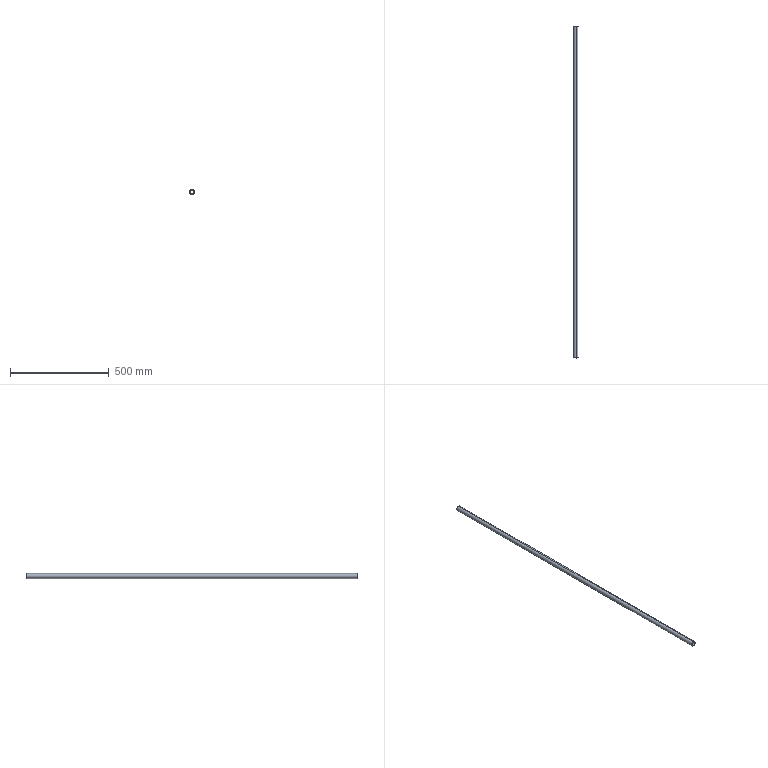Part | STEP file | PN_0046_Default<As Machined> | 1 solid | 6 faces | box 25.4 x 1683 x 25.4 mm | volume 334580 mm3 | cylinder 4 | plane 2 | commonest cylinder face diameters 19.8 x2 25.4 x2
STEP:
#1=CARTESIAN_POINT('',(0.,1683.,-9.9));
#2=VERTEX_POINT('',#1);
#3=CARTESIAN_POINT('',(0.,1683.,9.9));
#4=VERTEX_POINT('',#3);
#5=CARTESIAN_POINT('',(0.,1683.,0.));
#6=DIRECTION('',(0.,-1.,0.));
#7=AXIS2_PLACEMENT_3D('',#5,#6,$);
#8=CIRCLE('',#7,9.9);
#9=EDGE_CURVE('',#2,#4,#8,.F.);
#10=ORIENTED_EDGE('',*,*,#9,.T.);
#11=CARTESIAN_POINT('',(0.,0.,9.9));
#12=VERTEX_POINT('',#11);
#13=CARTESIAN_POINT('',(0.,1683.,9.9));
#14=DIRECTION('',(0.,-1.,0.));
#15=VECTOR('',#14,1.);
#16=LINE('',#13,#15);
#17=EDGE_CURVE('',#4,#12,#16,.T.);
#18=ORIENTED_EDGE('',*,*,#17,.T.);
#19=CARTESIAN_POINT('',(0.,0.,-9.9));
#20=VERTEX_POINT('',#19);
#21=CARTESIAN_POINT('',(0.,0.,0.));
#22=DIRECTION('',(0.,-1.,0.));
#23=AXIS2_PLACEMENT_3D('',#21,#22,$);
#24=CIRCLE('',#23,9.9);
#25=EDGE_CURVE('',#20,#12,#24,.F.);
#26=ORIENTED_EDGE('',*,*,#25,.F.);
#27=CARTESIAN_POINT('',(0.,1683.,-9.9));
#28=DIRECTION('',(0.,-1.,0.));
#29=VECTOR('',#28,1.);
#30=LINE('',#27,#29);
#31=EDGE_CURVE('',#2,#20,#30,.T.);
#32=ORIENTED_EDGE('',*,*,#31,.F.);
#33=EDGE_LOOP('',(#10,#18,#26,#32));
#34=FACE_OUTER_BOUND('',#33,.T.);
#35=CARTESIAN_POINT('',(0.,1683.,0.));
#36=DIRECTION('',(0.,-1.,0.));
#37=DIRECTION('',(0.,0.,1.));
#38=AXIS2_PLACEMENT_3D('',#35,#36,#37);
#39=CYLINDRICAL_SURFACE('',#38,9.9);
#40=ADVANCED_FACE('',(#34),#39,.F.);
#41=CARTESIAN_POINT('',(0.,1683.,-12.7));
#42=VERTEX_POINT('',#41);
#43=CARTESIAN_POINT('',(0.,1683.,12.7));
#44=VERTEX_POINT('',#43);
#45=CARTESIAN_POINT('',(0.,1683.,0.));
#46=DIRECTION('',(0.,1.,0.));
#47=AXIS2_PLACEMENT_3D('',#45,#46,$);
#48=CIRCLE('',#47,12.7);
#49=EDGE_CURVE('',#42,#44,#48,.T.);
#50=ORIENTED_EDGE('',*,*,#49,.T.);
#51=CARTESIAN_POINT('',(0.,1683.,0.));
#52=DIRECTION('',(0.,1.,0.));
#53=AXIS2_PLACEMENT_3D('',#51,#52,$);
#54=CIRCLE('',#53,12.7);
#55=EDGE_CURVE('',#44,#42,#54,.T.);
#56=ORIENTED_EDGE('',*,*,#55,.T.);
#57=EDGE_LOOP('',(#50,#56));
#58=FACE_OUTER_BOUND('',#57,.T.);
#59=ORIENTED_EDGE('',*,*,#9,.F.);
#60=CARTESIAN_POINT('',(0.,1683.,0.));
#61=DIRECTION('',(0.,1.,0.));
#62=AXIS2_PLACEMENT_3D('',#60,#61,$);
#63=CIRCLE('',#62,9.9);
#64=EDGE_CURVE('',#4,#2,#63,.T.);
#65=ORIENTED_EDGE('',*,*,#64,.F.);
#66=EDGE_LOOP('',(#59,#65));
#67=FACE_BOUND('',#66,.T.);
#68=CARTESIAN_POINT('',(0.,1683.,0.));
#69=DIRECTION('',(0.,1.,0.));
#70=DIRECTION('',(0.,0.,1.));
#71=AXIS2_PLACEMENT_3D('',#68,#69,#70);
#72=PLANE('',#71);
#73=ADVANCED_FACE('',(#58,#67),#72,.T.);
#74=ORIENTED_EDGE('',*,*,#17,.F.);
#75=ORIENTED_EDGE('',*,*,#64,.T.);
#76=ORIENTED_EDGE('',*,*,#31,.T.);
#77=CARTESIAN_POINT('',(0.,0.,0.));
#78=DIRECTION('',(0.,-1.,0.));
#79=AXIS2_PLACEMENT_3D('',#77,#78,$);
#80=CIRCLE('',#79,9.9);
#81=EDGE_CURVE('',#12,#20,#80,.F.);
#82=ORIENTED_EDGE('',*,*,#81,.F.);
#83=EDGE_LOOP('',(#74,#75,#76,#82));
#84=FACE_OUTER_BOUND('',#83,.T.);
#85=CARTESIAN_POINT('',(0.,1683.,0.));
#86=DIRECTION('',(0.,-1.,0.));
#87=DIRECTION('',(0.,0.,-1.));
#88=AXIS2_PLACEMENT_3D('',#85,#86,#87);
#89=CYLINDRICAL_SURFACE('',#88,9.9);
#90=ADVANCED_FACE('',(#84),#89,.F.);
#91=CARTESIAN_POINT('',(0.,0.,-12.7));
#92=VERTEX_POINT('',#91);
#93=CARTESIAN_POINT('',(0.,0.,12.7));
#94=VERTEX_POINT('',#93);
#95=CARTESIAN_POINT('',(0.,0.,0.));
#96=DIRECTION('',(0.,1.,0.));
#97=AXIS2_PLACEMENT_3D('',#95,#96,$);
#98=CIRCLE('',#97,12.7);
#99=EDGE_CURVE('',#92,#94,#98,.T.);
#100=ORIENTED_EDGE('',*,*,#99,.F.);
#101=CARTESIAN_POINT('',(0.,0.,0.));
#102=DIRECTION('',(0.,1.,0.));
#103=AXIS2_PLACEMENT_3D('',#101,#102,$);
#104=CIRCLE('',#103,12.7);
#105=EDGE_CURVE('',#94,#92,#104,.T.);
#106=ORIENTED_EDGE('',*,*,#105,.F.);
#107=EDGE_LOOP('',(#100,#106));
#108=FACE_OUTER_BOUND('',#107,.T.);
#109=ORIENTED_EDGE('',*,*,#25,.T.);
#110=ORIENTED_EDGE('',*,*,#81,.T.);
#111=EDGE_LOOP('',(#109,#110));
#112=FACE_BOUND('',#111,.T.);
#113=CARTESIAN_POINT('',(0.,0.,0.));
#114=DIRECTION('',(0.,1.,0.));
#115=DIRECTION('',(0.,0.,1.));
#116=AXIS2_PLACEMENT_3D('',#113,#114,#115);
#117=PLANE('',#116);
#118=ADVANCED_FACE('',(#108,#112),#117,.F.);
#119=CARTESIAN_POINT('',(0.,1683.,12.7));
#120=DIRECTION('',(0.,-1.,0.));
#121=VECTOR('',#120,1.);
#122=LINE('',#119,#121);
#123=EDGE_CURVE('',#44,#94,#122,.T.);
#124=ORIENTED_EDGE('',*,*,#123,.F.);
#125=ORIENTED_EDGE('',*,*,#49,.F.);
#126=CARTESIAN_POINT('',(0.,1683.,-12.7));
#127=DIRECTION('',(0.,-1.,0.));
#128=VECTOR('',#127,1.);
#129=LINE('',#126,#128);
#130=EDGE_CURVE('',#42,#92,#129,.T.);
#131=ORIENTED_EDGE('',*,*,#130,.T.);
#132=ORIENTED_EDGE('',*,*,#99,.T.);
#133=EDGE_LOOP('',(#124,#125,#131,#132));
#134=FACE_OUTER_BOUND('',#133,.T.);
#135=CARTESIAN_POINT('',(0.,1683.,0.));
#136=DIRECTION('',(0.,-1.,0.));
#137=DIRECTION('',(0.,0.,1.));
#138=AXIS2_PLACEMENT_3D('',#135,#136,#137);
#139=CYLINDRICAL_SURFACE('',#138,12.7);
#140=ADVANCED_FACE('',(#134),#139,.T.);
#141=ORIENTED_EDGE('',*,*,#55,.F.);
#142=ORIENTED_EDGE('',*,*,#123,.T.);
#143=ORIENTED_EDGE('',*,*,#105,.T.);
#144=ORIENTED_EDGE('',*,*,#130,.F.);
#145=EDGE_LOOP('',(#141,#142,#143,#144));
#146=FACE_OUTER_BOUND('',#145,.T.);
#147=CARTESIAN_POINT('',(0.,1683.,0.));
#148=DIRECTION('',(0.,-1.,0.));
#149=DIRECTION('',(0.,0.,-1.));
#150=AXIS2_PLACEMENT_3D('',#147,#148,#149);
#151=CYLINDRICAL_SURFACE('',#150,12.7);
#152=ADVANCED_FACE('',(#146),#151,.T.);
#153=CLOSED_SHELL('',(#40,#73,#90,#118,#140,#152));
#154=MANIFOLD_SOLID_BREP('',#153);
#155=(LENGTH_UNIT()NAMED_UNIT(*)SI_UNIT(.MILLI.,.METRE.));
#156=UNCERTAINTY_MEASURE_WITH_UNIT(LENGTH_MEASURE(0.005),#155,'','');
#157=(NAMED_UNIT(*)PLANE_ANGLE_UNIT()SI_UNIT($,.RADIAN.));
#158=(NAMED_UNIT(*)SI_UNIT($,.STERADIAN.)SOLID_ANGLE_UNIT());
#159=(GEOMETRIC_REPRESENTATION_CONTEXT(3)GLOBAL_UNCERTAINTY_ASSIGNED_CONTEXT((#156))GLOBAL_UNIT_ASSIGNED_CONTEXT((#155,#157,#158))REPRESENTATION_CONTEXT('',''));
#160=ADVANCED_BREP_SHAPE_REPRESENTATION('',(#154),#159);